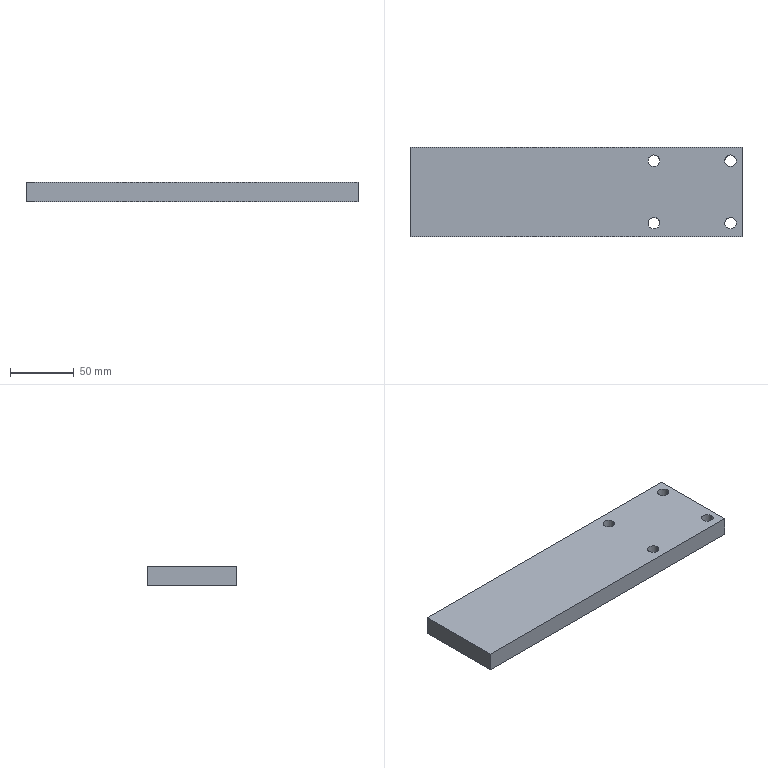Part | STEP file | Positioning_id466_x_t | 1 solid | 14 faces | box 260 x 70 x 15 mm | volume 269183 mm3 | cylinder 8 | plane 6 | commonest cylinder face diameters 9 x8
STEP:
#1=CARTESIAN_POINT('',(0.,0.,0.));
#2=DIRECTION('',(0.,0.,1.));
#3=DIRECTION('',(1.,0.,0.));
#4=AXIS2_PLACEMENT_3D('',#1,#2,#3);
#5=CARTESIAN_POINT('',(-826.502,-177.,373.532));
#6=VERTEX_POINT('',#5);
#7=CARTESIAN_POINT('',(-817.502,-177.,373.532));
#8=VERTEX_POINT('',#7);
#9=CARTESIAN_POINT('',(-822.002,-177.,373.532));
#10=DIRECTION('',(0.,0.,1.));
#11=DIRECTION('',(-1.,0.,0.));
#12=AXIS2_PLACEMENT_3D('',#9,#10,#11);
#13=CIRCLE('',#12,4.5);
#14=CARTESIAN_POINT('',(-822.002,-177.,293.532));
#15=DIRECTION('',(0.,0.,-1.));
#16=DIRECTION('',(1.,0.,0.));
#17=AXIS2_PLACEMENT_3D('',#14,#15,#16);
#18=CYLINDRICAL_SURFACE('',#17,4.5);
#19=CARTESIAN_POINT('',(3.142,-80.));
#20=DIRECTION('',(-1.,0.));
#21=VECTOR('',#20,1.);
#22=LINE('',#19,#21);
#23=(GEOMETRIC_REPRESENTATION_CONTEXT(2)PARAMETRIC_REPRESENTATION_CONTEXT()REPRESENTATION_CONTEXT('',''));
#24=DEFINITIONAL_REPRESENTATION('',(#22),#23);
#25=PCURVE('',#18,#24);
#26=CARTESIAN_POINT('',(-850.002,-164.,373.532));
#27=DIRECTION('',(0.,0.,1.));
#28=DIRECTION('',(0.,1.,0.));
#29=AXIS2_PLACEMENT_3D('',#26,#27,#28);
#30=PLANE('',#29);
#31=CARTESIAN_POINT('',(-13.,-28.));
#32=DIRECTION('',(0.,1.));
#33=AXIS2_PLACEMENT_2D('',#31,#32);
#34=CIRCLE('',#33,4.5);
#35=(GEOMETRIC_REPRESENTATION_CONTEXT(2)PARAMETRIC_REPRESENTATION_CONTEXT()REPRESENTATION_CONTEXT('',''));
#36=DEFINITIONAL_REPRESENTATION('',(#34),#35);
#37=PCURVE('',#30,#36);
#38=SURFACE_CURVE('',#13,(#25,#37),.PCURVE_S1.);
#39=EDGE_CURVE('',#6,#8,#38,.T.);
#40=ORIENTED_EDGE('',*,*,#39,.F.);
#41=CARTESIAN_POINT('',(-826.502,-177.,358.532));
#42=VERTEX_POINT('',#41);
#43=CARTESIAN_POINT('',(-826.502,-177.,358.532));
#44=DIRECTION('',(0.,0.,1.));
#45=VECTOR('',#44,1.);
#46=LINE('',#43,#45);
#47=CARTESIAN_POINT('',(3.142,-65.));
#48=DIRECTION('',(0.,-1.));
#49=VECTOR('',#48,1.);
#50=LINE('',#47,#49);
#51=(GEOMETRIC_REPRESENTATION_CONTEXT(2)PARAMETRIC_REPRESENTATION_CONTEXT()REPRESENTATION_CONTEXT('',''));
#52=DEFINITIONAL_REPRESENTATION('',(#50),#51);
#53=PCURVE('',#18,#52);
#54=CARTESIAN_POINT('',(-822.002,-177.,293.532));
#55=DIRECTION('',(0.,0.,-1.));
#56=DIRECTION('',(1.,0.,0.));
#57=AXIS2_PLACEMENT_3D('',#54,#55,#56);
#58=CYLINDRICAL_SURFACE('',#57,4.5);
#59=CARTESIAN_POINT('',(3.142,-65.));
#60=DIRECTION('',(0.,-1.));
#61=VECTOR('',#60,1.);
#62=LINE('',#59,#61);
#63=(GEOMETRIC_REPRESENTATION_CONTEXT(2)PARAMETRIC_REPRESENTATION_CONTEXT()REPRESENTATION_CONTEXT('',''));
#64=DEFINITIONAL_REPRESENTATION('',(#62),#63);
#65=PCURVE('',#58,#64);
#66=SURFACE_CURVE('',#46,(#53,#65),.PCURVE_S1.);
#67=EDGE_CURVE('',#42,#6,#66,.T.);
#68=ORIENTED_EDGE('',*,*,#67,.F.);
#69=CARTESIAN_POINT('',(-817.502,-177.,358.532));
#70=VERTEX_POINT('',#69);
#71=CARTESIAN_POINT('',(-822.002,-177.,358.532));
#72=DIRECTION('',(0.,0.,-1.));
#73=DIRECTION('',(-1.,0.,0.));
#74=AXIS2_PLACEMENT_3D('',#71,#72,#73);
#75=CIRCLE('',#74,4.5);
#76=CARTESIAN_POINT('',(-3.142,-65.));
#77=DIRECTION('',(1.,0.));
#78=VECTOR('',#77,1.);
#79=LINE('',#76,#78);
#80=(GEOMETRIC_REPRESENTATION_CONTEXT(2)PARAMETRIC_REPRESENTATION_CONTEXT()REPRESENTATION_CONTEXT('',''));
#81=DEFINITIONAL_REPRESENTATION('',(#79),#80);
#82=PCURVE('',#18,#81);
#83=CARTESIAN_POINT('',(-850.002,-164.,358.532));
#84=DIRECTION('',(0.,0.,-1.));
#85=DIRECTION('',(0.,-1.,0.));
#86=AXIS2_PLACEMENT_3D('',#83,#84,#85);
#87=PLANE('',#86);
#88=CARTESIAN_POINT('',(13.,-28.));
#89=DIRECTION('',(0.,1.));
#90=AXIS2_PLACEMENT_2D('',#88,#89);
#91=CIRCLE('',#90,4.5);
#92=(GEOMETRIC_REPRESENTATION_CONTEXT(2)PARAMETRIC_REPRESENTATION_CONTEXT()REPRESENTATION_CONTEXT('',''));
#93=DEFINITIONAL_REPRESENTATION('',(#91),#92);
#94=PCURVE('',#87,#93);
#95=SURFACE_CURVE('',#75,(#82,#94),.PCURVE_S1.);
#96=EDGE_CURVE('',#70,#42,#95,.T.);
#97=ORIENTED_EDGE('',*,*,#96,.F.);
#98=CARTESIAN_POINT('',(-817.502,-177.,358.532));
#99=DIRECTION('',(0.,0.,-1.));
#100=VECTOR('',#99,1.);
#101=LINE('',#98,#100);
#102=CARTESIAN_POINT('',(0.,-65.));
#103=DIRECTION('',(0.,1.));
#104=VECTOR('',#103,1.);
#105=LINE('',#102,#104);
#106=(GEOMETRIC_REPRESENTATION_CONTEXT(2)PARAMETRIC_REPRESENTATION_CONTEXT()REPRESENTATION_CONTEXT('',''));
#107=DEFINITIONAL_REPRESENTATION('',(#105),#106);
#108=PCURVE('',#18,#107);
#109=CARTESIAN_POINT('',(6.283,-65.));
#110=DIRECTION('',(0.,1.));
#111=VECTOR('',#110,1.);
#112=LINE('',#109,#111);
#113=(GEOMETRIC_REPRESENTATION_CONTEXT(2)PARAMETRIC_REPRESENTATION_CONTEXT()REPRESENTATION_CONTEXT('',''));
#114=DEFINITIONAL_REPRESENTATION('',(#112),#113);
#115=PCURVE('',#58,#114);
#116=SURFACE_CURVE('',#101,(#108,#115),.PCURVE_S1.);
#117=EDGE_CURVE('',#8,#70,#116,.T.);
#118=ORIENTED_EDGE('',*,*,#117,.F.);
#119=EDGE_LOOP('',(#40,#68,#97,#118));
#120=FACE_BOUND('',#119,.F.);
#121=ADVANCED_FACE('',(#120),#18,.F.);
#122=CARTESIAN_POINT('',(-826.502,-226.,373.532));
#123=VERTEX_POINT('',#122);
#124=CARTESIAN_POINT('',(-817.502,-226.,373.532));
#125=VERTEX_POINT('',#124);
#126=CARTESIAN_POINT('',(-822.002,-226.,373.532));
#127=DIRECTION('',(0.,0.,1.));
#128=DIRECTION('',(-1.,0.,0.));
#129=AXIS2_PLACEMENT_3D('',#126,#127,#128);
#130=CIRCLE('',#129,4.5);
#131=CARTESIAN_POINT('',(-822.002,-226.,293.532));
#132=DIRECTION('',(0.,0.,-1.));
#133=DIRECTION('',(1.,0.,0.));
#134=AXIS2_PLACEMENT_3D('',#131,#132,#133);
#135=CYLINDRICAL_SURFACE('',#134,4.5);
#136=CARTESIAN_POINT('',(3.142,-80.));
#137=DIRECTION('',(-1.,0.));
#138=VECTOR('',#137,1.);
#139=LINE('',#136,#138);
#140=(GEOMETRIC_REPRESENTATION_CONTEXT(2)PARAMETRIC_REPRESENTATION_CONTEXT()REPRESENTATION_CONTEXT('',''));
#141=DEFINITIONAL_REPRESENTATION('',(#139),#140);
#142=PCURVE('',#135,#141);
#143=CARTESIAN_POINT('',(-62.,-28.));
#144=DIRECTION('',(0.,1.));
#145=AXIS2_PLACEMENT_2D('',#143,#144);
#146=CIRCLE('',#145,4.5);
#147=(GEOMETRIC_REPRESENTATION_CONTEXT(2)PARAMETRIC_REPRESENTATION_CONTEXT()REPRESENTATION_CONTEXT('',''));
#148=DEFINITIONAL_REPRESENTATION('',(#146),#147);
#149=PCURVE('',#30,#148);
#150=SURFACE_CURVE('',#130,(#142,#149),.PCURVE_S1.);
#151=EDGE_CURVE('',#123,#125,#150,.T.);
#152=ORIENTED_EDGE('',*,*,#151,.F.);
#153=CARTESIAN_POINT('',(-826.502,-226.,358.532));
#154=VERTEX_POINT('',#153);
#155=CARTESIAN_POINT('',(-826.502,-226.,358.532));
#156=DIRECTION('',(0.,0.,-1.));
#157=VECTOR('',#156,1.);
#158=LINE('',#155,#157);
#159=CARTESIAN_POINT('',(3.142,-65.));
#160=DIRECTION('',(0.,1.));
#161=VECTOR('',#160,1.);
#162=LINE('',#159,#161);
#163=(GEOMETRIC_REPRESENTATION_CONTEXT(2)PARAMETRIC_REPRESENTATION_CONTEXT()REPRESENTATION_CONTEXT('',''));
#164=DEFINITIONAL_REPRESENTATION('',(#162),#163);
#165=PCURVE('',#135,#164);
#166=CARTESIAN_POINT('',(-822.002,-226.,293.532));
#167=DIRECTION('',(0.,0.,-1.));
#168=DIRECTION('',(1.,0.,0.));
#169=AXIS2_PLACEMENT_3D('',#166,#167,#168);
#170=CYLINDRICAL_SURFACE('',#169,4.5);
#171=CARTESIAN_POINT('',(3.142,-65.));
#172=DIRECTION('',(0.,1.));
#173=VECTOR('',#172,1.);
#174=LINE('',#171,#173);
#175=(GEOMETRIC_REPRESENTATION_CONTEXT(2)PARAMETRIC_REPRESENTATION_CONTEXT()REPRESENTATION_CONTEXT('',''));
#176=DEFINITIONAL_REPRESENTATION('',(#174),#175);
#177=PCURVE('',#170,#176);
#178=SURFACE_CURVE('',#158,(#165,#177),.PCURVE_S1.);
#179=EDGE_CURVE('',#123,#154,#178,.T.);
#180=ORIENTED_EDGE('',*,*,#179,.T.);
#181=CARTESIAN_POINT('',(-817.502,-226.,358.532));
#182=VERTEX_POINT('',#181);
#183=CARTESIAN_POINT('',(-822.002,-226.,358.532));
#184=DIRECTION('',(0.,0.,-1.));
#185=DIRECTION('',(-1.,0.,0.));
#186=AXIS2_PLACEMENT_3D('',#183,#184,#185);
#187=CIRCLE('',#186,4.5);
#188=CARTESIAN_POINT('',(-3.142,-65.));
#189=DIRECTION('',(1.,0.));
#190=VECTOR('',#189,1.);
#191=LINE('',#188,#190);
#192=(GEOMETRIC_REPRESENTATION_CONTEXT(2)PARAMETRIC_REPRESENTATION_CONTEXT()REPRESENTATION_CONTEXT('',''));
#193=DEFINITIONAL_REPRESENTATION('',(#191),#192);
#194=PCURVE('',#135,#193);
#195=CARTESIAN_POINT('',(62.,-28.));
#196=DIRECTION('',(0.,1.));
#197=AXIS2_PLACEMENT_2D('',#195,#196);
#198=CIRCLE('',#197,4.5);
#199=(GEOMETRIC_REPRESENTATION_CONTEXT(2)PARAMETRIC_REPRESENTATION_CONTEXT()REPRESENTATION_CONTEXT('',''));
#200=DEFINITIONAL_REPRESENTATION('',(#198),#199);
#201=PCURVE('',#87,#200);
#202=SURFACE_CURVE('',#187,(#194,#201),.PCURVE_S1.);
#203=EDGE_CURVE('',#182,#154,#202,.T.);
#204=ORIENTED_EDGE('',*,*,#203,.F.);
#205=CARTESIAN_POINT('',(-817.502,-226.,358.532));
#206=DIRECTION('',(0.,0.,1.));
#207=VECTOR('',#206,1.);
#208=LINE('',#205,#207);
#209=CARTESIAN_POINT('',(0.,-65.));
#210=DIRECTION('',(0.,-1.));
#211=VECTOR('',#210,1.);
#212=LINE('',#209,#211);
#213=(GEOMETRIC_REPRESENTATION_CONTEXT(2)PARAMETRIC_REPRESENTATION_CONTEXT()REPRESENTATION_CONTEXT('',''));
#214=DEFINITIONAL_REPRESENTATION('',(#212),#213);
#215=PCURVE('',#135,#214);
#216=CARTESIAN_POINT('',(6.283,-65.));
#217=DIRECTION('',(0.,-1.));
#218=VECTOR('',#217,1.);
#219=LINE('',#216,#218);
#220=(GEOMETRIC_REPRESENTATION_CONTEXT(2)PARAMETRIC_REPRESENTATION_CONTEXT()REPRESENTATION_CONTEXT('',''));
#221=DEFINITIONAL_REPRESENTATION('',(#219),#220);
#222=PCURVE('',#170,#221);
#223=SURFACE_CURVE('',#208,(#215,#222),.PCURVE_S1.);
#224=EDGE_CURVE('',#182,#125,#223,.T.);
#225=ORIENTED_EDGE('',*,*,#224,.T.);
#226=EDGE_LOOP('',(#152,#180,#204,#225));
#227=FACE_BOUND('',#226,.F.);
#228=ADVANCED_FACE('',(#227),#135,.F.);
#229=CARTESIAN_POINT('',(-766.502,-226.,373.532));
#230=VERTEX_POINT('',#229);
#231=CARTESIAN_POINT('',(-757.502,-226.,373.532));
#232=VERTEX_POINT('',#231);
#233=CARTESIAN_POINT('',(-762.002,-226.,373.532));
#234=DIRECTION('',(0.,0.,1.));
#235=DIRECTION('',(-1.,0.,0.));
#236=AXIS2_PLACEMENT_3D('',#233,#234,#235);
#237=CIRCLE('',#236,4.5);
#238=CARTESIAN_POINT('',(-762.002,-226.,293.532));
#239=DIRECTION('',(0.,0.,-1.));
#240=DIRECTION('',(1.,0.,0.));
#241=AXIS2_PLACEMENT_3D('',#238,#239,#240);
#242=CYLINDRICAL_SURFACE('',#241,4.5);
#243=CARTESIAN_POINT('',(3.142,-80.));
#244=DIRECTION('',(-1.,0.));
#245=VECTOR('',#244,1.);
#246=LINE('',#243,#245);
#247=(GEOMETRIC_REPRESENTATION_CONTEXT(2)PARAMETRIC_REPRESENTATION_CONTEXT()REPRESENTATION_CONTEXT('',''));
#248=DEFINITIONAL_REPRESENTATION('',(#246),#247);
#249=PCURVE('',#242,#248);
#250=CARTESIAN_POINT('',(-62.,-88.));
#251=DIRECTION('',(0.,1.));
#252=AXIS2_PLACEMENT_2D('',#250,#251);
#253=CIRCLE('',#252,4.5);
#254=(GEOMETRIC_REPRESENTATION_CONTEXT(2)PARAMETRIC_REPRESENTATION_CONTEXT()REPRESENTATION_CONTEXT('',''));
#255=DEFINITIONAL_REPRESENTATION('',(#253),#254);
#256=PCURVE('',#30,#255);
#257=SURFACE_CURVE('',#237,(#249,#256),.PCURVE_S1.);
#258=EDGE_CURVE('',#230,#232,#257,.T.);
#259=ORIENTED_EDGE('',*,*,#258,.F.);
#260=CARTESIAN_POINT('',(-766.502,-226.,358.532));
#261=VERTEX_POINT('',#260);
#262=CARTESIAN_POINT('',(-766.502,-226.,358.532));
#263=DIRECTION('',(0.,0.,1.));
#264=VECTOR('',#263,1.);
#265=LINE('',#262,#264);
#266=CARTESIAN_POINT('',(3.142,-65.));
#267=DIRECTION('',(0.,-1.));
#268=VECTOR('',#267,1.);
#269=LINE('',#266,#268);
#270=(GEOMETRIC_REPRESENTATION_CONTEXT(2)PARAMETRIC_REPRESENTATION_CONTEXT()REPRESENTATION_CONTEXT('',''));
#271=DEFINITIONAL_REPRESENTATION('',(#269),#270);
#272=PCURVE('',#242,#271);
#273=CARTESIAN_POINT('',(-762.002,-226.,293.532));
#274=DIRECTION('',(0.,0.,-1.));
#275=DIRECTION('',(1.,0.,0.));
#276=AXIS2_PLACEMENT_3D('',#273,#274,#275);
#277=CYLINDRICAL_SURFACE('',#276,4.5);
#278=CARTESIAN_POINT('',(3.142,-65.));
#279=DIRECTION('',(0.,-1.));
#280=VECTOR('',#279,1.);
#281=LINE('',#278,#280);
#282=(GEOMETRIC_REPRESENTATION_CONTEXT(2)PARAMETRIC_REPRESENTATION_CONTEXT()REPRESENTATION_CONTEXT('',''));
#283=DEFINITIONAL_REPRESENTATION('',(#281),#282);
#284=PCURVE('',#277,#283);
#285=SURFACE_CURVE('',#265,(#272,#284),.PCURVE_S1.);
#286=EDGE_CURVE('',#261,#230,#285,.T.);
#287=ORIENTED_EDGE('',*,*,#286,.F.);
#288=CARTESIAN_POINT('',(-757.502,-226.,358.532));
#289=VERTEX_POINT('',#288);
#290=CARTESIAN_POINT('',(-762.002,-226.,358.532));
#291=DIRECTION('',(0.,0.,-1.));
#292=DIRECTION('',(-1.,0.,0.));
#293=AXIS2_PLACEMENT_3D('',#290,#291,#292);
#294=CIRCLE('',#293,4.5);
#295=CARTESIAN_POINT('',(-3.142,-65.));
#296=DIRECTION('',(1.,0.));
#297=VECTOR('',#296,1.);
#298=LINE('',#295,#297);
#299=(GEOMETRIC_REPRESENTATION_CONTEXT(2)PARAMETRIC_REPRESENTATION_CONTEXT()REPRESENTATION_CONTEXT('',''));
#300=DEFINITIONAL_REPRESENTATION('',(#298),#299);
#301=PCURVE('',#242,#300);
#302=CARTESIAN_POINT('',(62.,-88.));
#303=DIRECTION('',(0.,1.));
#304=AXIS2_PLACEMENT_2D('',#302,#303);
#305=CIRCLE('',#304,4.5);
#306=(GEOMETRIC_REPRESENTATION_CONTEXT(2)PARAMETRIC_REPRESENTATION_CONTEXT()REPRESENTATION_CONTEXT('',''));
#307=DEFINITIONAL_REPRESENTATION('',(#305),#306);
#308=PCURVE('',#87,#307);
#309=SURFACE_CURVE('',#294,(#301,#308),.PCURVE_S1.);
#310=EDGE_CURVE('',#289,#261,#309,.T.);
#311=ORIENTED_EDGE('',*,*,#310,.F.);
#312=CARTESIAN_POINT('',(-757.502,-226.,358.532));
#313=DIRECTION('',(0.,0.,-1.));
#314=VECTOR('',#313,1.);
#315=LINE('',#312,#314);
#316=CARTESIAN_POINT('',(0.,-65.));
#317=DIRECTION('',(0.,1.));
#318=VECTOR('',#317,1.);
#319=LINE('',#316,#318);
#320=(GEOMETRIC_REPRESENTATION_CONTEXT(2)PARAMETRIC_REPRESENTATION_CONTEXT()REPRESENTATION_CONTEXT('',''));
#321=DEFINITIONAL_REPRESENTATION('',(#319),#320);
#322=PCURVE('',#242,#321);
#323=CARTESIAN_POINT('',(6.283,-65.));
#324=DIRECTION('',(0.,1.));
#325=VECTOR('',#324,1.);
#326=LINE('',#323,#325);
#327=(GEOMETRIC_REPRESENTATION_CONTEXT(2)PARAMETRIC_REPRESENTATION_CONTEXT()REPRESENTATION_CONTEXT('',''));
#328=DEFINITIONAL_REPRESENTATION('',(#326),#327);
#329=PCURVE('',#277,#328);
#330=SURFACE_CURVE('',#315,(#322,#329),.PCURVE_S1.);
#331=EDGE_CURVE('',#232,#289,#330,.T.);
#332=ORIENTED_EDGE('',*,*,#331,.F.);
#333=EDGE_LOOP('',(#259,#287,#311,#332));
#334=FACE_BOUND('',#333,.F.);
#335=ADVANCED_FACE('',(#334),#242,.F.);
#336=CARTESIAN_POINT('',(-766.502,-177.,373.532));
#337=VERTEX_POINT('',#336);
#338=CARTESIAN_POINT('',(-757.502,-177.,373.532));
#339=VERTEX_POINT('',#338);
#340=CARTESIAN_POINT('',(-762.002,-177.,373.532));
#341=DIRECTION('',(0.,0.,1.));
#342=DIRECTION('',(-1.,0.,0.));
#343=AXIS2_PLACEMENT_3D('',#340,#341,#342);
#344=CIRCLE('',#343,4.5);
#345=CARTESIAN_POINT('',(-762.002,-177.,293.532));
#346=DIRECTION('',(0.,0.,-1.));
#347=DIRECTION('',(1.,0.,0.));
#348=AXIS2_PLACEMENT_3D('',#345,#346,#347);
#349=CYLINDRICAL_SURFACE('',#348,4.5);
#350=CARTESIAN_POINT('',(3.142,-80.));
#351=DIRECTION('',(-1.,0.));
#352=VECTOR('',#351,1.);
#353=LINE('',#350,#352);
#354=(GEOMETRIC_REPRESENTATION_CONTEXT(2)PARAMETRIC_REPRESENTATION_CONTEXT()REPRESENTATION_CONTEXT('',''));
#355=DEFINITIONAL_REPRESENTATION('',(#353),#354);
#356=PCURVE('',#349,#355);
#357=CARTESIAN_POINT('',(-13.,-88.));
#358=DIRECTION('',(0.,1.));
#359=AXIS2_PLACEMENT_2D('',#357,#358);
#360=CIRCLE('',#359,4.5);
#361=(GEOMETRIC_REPRESENTATION_CONTEXT(2)PARAMETRIC_REPRESENTATION_CONTEXT()REPRESENTATION_CONTEXT('',''));
#362=DEFINITIONAL_REPRESENTATION('',(#360),#361);
#363=PCURVE('',#30,#362);
#364=SURFACE_CURVE('',#344,(#356,#363),.PCURVE_S1.);
#365=EDGE_CURVE('',#337,#339,#364,.T.);
#366=ORIENTED_EDGE('',*,*,#365,.F.);
#367=CARTESIAN_POINT('',(-766.502,-177.,358.532));
#368=VERTEX_POINT('',#367);
#369=CARTESIAN_POINT('',(-766.502,-177.,358.532));
#370=DIRECTION('',(0.,0.,-1.));
#371=VECTOR('',#370,1.);
#372=LINE('',#369,#371);
#373=CARTESIAN_POINT('',(3.142,-65.));
#374=DIRECTION('',(0.,1.));
#375=VECTOR('',#374,1.);
#376=LINE('',#373,#375);
#377=(GEOMETRIC_REPRESENTATION_CONTEXT(2)PARAMETRIC_REPRESENTATION_CONTEXT()REPRESENTATION_CONTEXT('',''));
#378=DEFINITIONAL_REPRESENTATION('',(#376),#377);
#379=PCURVE('',#349,#378);
#380=CARTESIAN_POINT('',(-762.002,-177.,293.532));
#381=DIRECTION('',(0.,0.,-1.));
#382=DIRECTION('',(1.,0.,0.));
#383=AXIS2_PLACEMENT_3D('',#380,#381,#382);
#384=CYLINDRICAL_SURFACE('',#383,4.5);
#385=CARTESIAN_POINT('',(3.142,-65.));
#386=DIRECTION('',(0.,1.));
#387=VECTOR('',#386,1.);
#388=LINE('',#385,#387);
#389=(GEOMETRIC_REPRESENTATION_CONTEXT(2)PARAMETRIC_REPRESENTATION_CONTEXT()REPRESENTATION_CONTEXT('',''));
#390=DEFINITIONAL_REPRESENTATION('',(#388),#389);
#391=PCURVE('',#384,#390);
#392=SURFACE_CURVE('',#372,(#379,#391),.PCURVE_S1.);
#393=EDGE_CURVE('',#337,#368,#392,.T.);
#394=ORIENTED_EDGE('',*,*,#393,.T.);
#395=CARTESIAN_POINT('',(-757.502,-177.,358.532));
#396=VERTEX_POINT('',#395);
#397=CARTESIAN_POINT('',(-762.002,-177.,358.532));
#398=DIRECTION('',(0.,0.,-1.));
#399=DIRECTION('',(-1.,0.,0.));
#400=AXIS2_PLACEMENT_3D('',#397,#398,#399);
#401=CIRCLE('',#400,4.5);
#402=CARTESIAN_POINT('',(-3.142,-65.));
#403=DIRECTION('',(1.,0.));
#404=VECTOR('',#403,1.);
#405=LINE('',#402,#404);
#406=(GEOMETRIC_REPRESENTATION_CONTEXT(2)PARAMETRIC_REPRESENTATION_CONTEXT()REPRESENTATION_CONTEXT('',''));
#407=DEFINITIONAL_REPRESENTATION('',(#405),#406);
#408=PCURVE('',#349,#407);
#409=CARTESIAN_POINT('',(13.,-88.));
#410=DIRECTION('',(0.,1.));
#411=AXIS2_PLACEMENT_2D('',#409,#410);
#412=CIRCLE('',#411,4.5);
#413=(GEOMETRIC_REPRESENTATION_CONTEXT(2)PARAMETRIC_REPRESENTATION_CONTEXT()REPRESENTATION_CONTEXT('',''));
#414=DEFINITIONAL_REPRESENTATION('',(#412),#413);
#415=PCURVE('',#87,#414);
#416=SURFACE_CURVE('',#401,(#408,#415),.PCURVE_S1.);
#417=EDGE_CURVE('',#396,#368,#416,.T.);
#418=ORIENTED_EDGE('',*,*,#417,.F.);
#419=CARTESIAN_POINT('',(-757.502,-177.,358.532));
#420=DIRECTION('',(0.,0.,1.));
#421=VECTOR('',#420,1.);
#422=LINE('',#419,#421);
#423=CARTESIAN_POINT('',(0.,-65.));
#424=DIRECTION('',(0.,-1.));
#425=VECTOR('',#424,1.);
#426=LINE('',#423,#425);
#427=(GEOMETRIC_REPRESENTATION_CONTEXT(2)PARAMETRIC_REPRESENTATION_CONTEXT()REPRESENTATION_CONTEXT('',''));
#428=DEFINITIONAL_REPRESENTATION('',(#426),#427);
#429=PCURVE('',#349,#428);
#430=CARTESIAN_POINT('',(6.283,-65.));
#431=DIRECTION('',(0.,-1.));
#432=VECTOR('',#431,1.);
#433=LINE('',#430,#432);
#434=(GEOMETRIC_REPRESENTATION_CONTEXT(2)PARAMETRIC_REPRESENTATION_CONTEXT()REPRESENTATION_CONTEXT('',''));
#435=DEFINITIONAL_REPRESENTATION('',(#433),#434);
#436=PCURVE('',#384,#435);
#437=SURFACE_CURVE('',#422,(#429,#436),.PCURVE_S1.);
#438=EDGE_CURVE('',#396,#339,#437,.T.);
#439=ORIENTED_EDGE('',*,*,#438,.T.);
#440=EDGE_LOOP('',(#366,#394,#418,#439));
#441=FACE_BOUND('',#440,.F.);
#442=ADVANCED_FACE('',(#441),#349,.F.);
#443=CARTESIAN_POINT('',(-1013.002,-236.5,358.532));
#444=VERTEX_POINT('',#443);
#445=CARTESIAN_POINT('',(-1013.002,-236.5,373.532));
#446=VERTEX_POINT('',#445);
#447=CARTESIAN_POINT('',(-1013.002,-236.5,358.532));
#448=DIRECTION('',(0.,0.,1.));
#449=VECTOR('',#448,1.);
#450=LINE('',#447,#449);
#451=CARTESIAN_POINT('',(-1013.002,95.25,13.032));
#452=DIRECTION('',(1.,0.,0.));
#453=DIRECTION('',(0.,-1.,0.));
#454=AXIS2_PLACEMENT_3D('',#451,#452,#453);
#455=PLANE('',#454);
#456=CARTESIAN_POINT('',(331.75,-345.5));
#457=DIRECTION('',(0.,-1.));
#458=VECTOR('',#457,1.);
#459=LINE('',#456,#458);
#460=(GEOMETRIC_REPRESENTATION_CONTEXT(2)PARAMETRIC_REPRESENTATION_CONTEXT()REPRESENTATION_CONTEXT('',''));
#461=DEFINITIONAL_REPRESENTATION('',(#459),#460);
#462=PCURVE('',#455,#461);
#463=CARTESIAN_POINT('',(-850.002,-236.5,388.532));
#464=DIRECTION('',(0.,-1.,0.));
#465=DIRECTION('',(-1.,0.,0.));
#466=AXIS2_PLACEMENT_3D('',#463,#464,#465);
#467=PLANE('',#466);
#468=CARTESIAN_POINT('',(163.,30.));
#469=DIRECTION('',(0.,-1.));
#470=VECTOR('',#469,1.);
#471=LINE('',#468,#470);
#472=(GEOMETRIC_REPRESENTATION_CONTEXT(2)PARAMETRIC_REPRESENTATION_CONTEXT()REPRESENTATION_CONTEXT('',''));
#473=DEFINITIONAL_REPRESENTATION('',(#471),#472);
#474=PCURVE('',#467,#473);
#475=SURFACE_CURVE('',#450,(#462,#474),.PCURVE_S1.);
#476=EDGE_CURVE('',#444,#446,#475,.T.);
#477=ORIENTED_EDGE('',*,*,#476,.T.);
#478=CARTESIAN_POINT('',(-1013.002,-166.5,373.532));
#479=VERTEX_POINT('',#478);
#480=CARTESIAN_POINT('',(-1013.002,-236.5,373.532));
#481=DIRECTION('',(0.,1.,0.));
#482=VECTOR('',#481,1.);
#483=LINE('',#480,#482);
#484=CARTESIAN_POINT('',(331.75,-360.5));
#485=DIRECTION('',(-1.,0.));
#486=VECTOR('',#485,1.);
#487=LINE('',#484,#486);
#488=(GEOMETRIC_REPRESENTATION_CONTEXT(2)PARAMETRIC_REPRESENTATION_CONTEXT()REPRESENTATION_CONTEXT('',''));
#489=DEFINITIONAL_REPRESENTATION('',(#487),#488);
#490=PCURVE('',#455,#489);
#491=CARTESIAN_POINT('',(-72.5,163.));
#492=DIRECTION('',(1.,0.));
#493=VECTOR('',#492,1.);
#494=LINE('',#491,#493);
#495=(GEOMETRIC_REPRESENTATION_CONTEXT(2)PARAMETRIC_REPRESENTATION_CONTEXT()REPRESENTATION_CONTEXT('',''));
#496=DEFINITIONAL_REPRESENTATION('',(#494),#495);
#497=PCURVE('',#30,#496);
#498=SURFACE_CURVE('',#483,(#490,#497),.PCURVE_S1.);
#499=EDGE_CURVE('',#446,#479,#498,.T.);
#500=ORIENTED_EDGE('',*,*,#499,.T.);
#501=CARTESIAN_POINT('',(-1013.002,-166.5,358.532));
#502=VERTEX_POINT('',#501);
#503=CARTESIAN_POINT('',(-1013.002,-166.5,373.532));
#504=DIRECTION('',(0.,0.,-1.));
#505=VECTOR('',#504,1.);
#506=LINE('',#503,#505);
#507=CARTESIAN_POINT('',(261.75,-360.5));
#508=DIRECTION('',(0.,1.));
#509=VECTOR('',#508,1.);
#510=LINE('',#507,#509);
#511=(GEOMETRIC_REPRESENTATION_CONTEXT(2)PARAMETRIC_REPRESENTATION_CONTEXT()REPRESENTATION_CONTEXT('',''));
#512=DEFINITIONAL_REPRESENTATION('',(#510),#511);
#513=PCURVE('',#455,#512);
#514=CARTESIAN_POINT('',(-850.002,-166.5,388.532));
#515=DIRECTION('',(0.,1.,0.));
#516=DIRECTION('',(1.,0.,0.));
#517=AXIS2_PLACEMENT_3D('',#514,#515,#516);
#518=PLANE('',#517);
#519=CARTESIAN_POINT('',(-163.,15.));
#520=DIRECTION('',(0.,1.));
#521=VECTOR('',#520,1.);
#522=LINE('',#519,#521);
#523=(GEOMETRIC_REPRESENTATION_CONTEXT(2)PARAMETRIC_REPRESENTATION_CONTEXT()REPRESENTATION_CONTEXT('',''));
#524=DEFINITIONAL_REPRESENTATION('',(#522),#523);
#525=PCURVE('',#518,#524);
#526=SURFACE_CURVE('',#506,(#513,#525),.PCURVE_S1.);
#527=EDGE_CURVE('',#479,#502,#526,.T.);
#528=ORIENTED_EDGE('',*,*,#527,.T.);
#529=CARTESIAN_POINT('',(-1013.002,-166.5,358.532));
#530=DIRECTION('',(0.,-1.,0.));
#531=VECTOR('',#530,1.);
#532=LINE('',#529,#531);
#533=CARTESIAN_POINT('',(261.75,-345.5));
#534=DIRECTION('',(1.,0.));
#535=VECTOR('',#534,1.);
#536=LINE('',#533,#535);
#537=(GEOMETRIC_REPRESENTATION_CONTEXT(2)PARAMETRIC_REPRESENTATION_CONTEXT()REPRESENTATION_CONTEXT('',''));
#538=DEFINITIONAL_REPRESENTATION('',(#536),#537);
#539=PCURVE('',#455,#538);
#540=CARTESIAN_POINT('',(2.5,163.));
#541=DIRECTION('',(1.,0.));
#542=VECTOR('',#541,1.);
#543=LINE('',#540,#542);
#544=(GEOMETRIC_REPRESENTATION_CONTEXT(2)PARAMETRIC_REPRESENTATION_CONTEXT()REPRESENTATION_CONTEXT('',''));
#545=DEFINITIONAL_REPRESENTATION('',(#543),#544);
#546=PCURVE('',#87,#545);
#547=SURFACE_CURVE('',#532,(#539,#546),.PCURVE_S1.);
#548=EDGE_CURVE('',#502,#444,#547,.T.);
#549=ORIENTED_EDGE('',*,*,#548,.T.);
#550=EDGE_LOOP('',(#477,#500,#528,#549));
#551=FACE_BOUND('',#550,.T.);
#552=ADVANCED_FACE('',(#551),#455,.F.);
#553=CARTESIAN_POINT('',(-753.002,-166.5,373.532));
#554=VERTEX_POINT('',#553);
#555=CARTESIAN_POINT('',(-753.002,-166.5,358.532));
#556=VERTEX_POINT('',#555);
#557=CARTESIAN_POINT('',(-753.002,-166.5,373.532));
#558=DIRECTION('',(0.,0.,-1.));
#559=VECTOR('',#558,1.);
#560=LINE('',#557,#559);
#561=CARTESIAN_POINT('',(-753.002,-164.,388.532));
#562=DIRECTION('',(1.,0.,0.));
#563=DIRECTION('',(0.,-1.,0.));
#564=AXIS2_PLACEMENT_3D('',#561,#562,#563);
#565=PLANE('',#564);
#566=CARTESIAN_POINT('',(2.5,15.));
#567=DIRECTION('',(0.,1.));
#568=VECTOR('',#567,1.);
#569=LINE('',#566,#568);
#570=(GEOMETRIC_REPRESENTATION_CONTEXT(2)PARAMETRIC_REPRESENTATION_CONTEXT()REPRESENTATION_CONTEXT('',''));
#571=DEFINITIONAL_REPRESENTATION('',(#569),#570);
#572=PCURVE('',#565,#571);
#573=CARTESIAN_POINT('',(97.,15.));
#574=DIRECTION('',(0.,1.));
#575=VECTOR('',#574,1.);
#576=LINE('',#573,#575);
#577=(GEOMETRIC_REPRESENTATION_CONTEXT(2)PARAMETRIC_REPRESENTATION_CONTEXT()REPRESENTATION_CONTEXT('',''));
#578=DEFINITIONAL_REPRESENTATION('',(#576),#577);
#579=PCURVE('',#518,#578);
#580=SURFACE_CURVE('',#560,(#572,#579),.PCURVE_S1.);
#581=EDGE_CURVE('',#554,#556,#580,.T.);
#582=ORIENTED_EDGE('',*,*,#581,.F.);
#583=CARTESIAN_POINT('',(-753.002,-236.5,373.532));
#584=VERTEX_POINT('',#583);
#585=CARTESIAN_POINT('',(-753.002,-166.5,373.532));
#586=DIRECTION('',(0.,-1.,0.));
#587=VECTOR('',#586,1.);
#588=LINE('',#585,#587);
#589=CARTESIAN_POINT('',(2.5,15.));
#590=DIRECTION('',(1.,0.));
#591=VECTOR('',#590,1.);
#592=LINE('',#589,#591);
#593=(GEOMETRIC_REPRESENTATION_CONTEXT(2)PARAMETRIC_REPRESENTATION_CONTEXT()REPRESENTATION_CONTEXT('',''));
#594=DEFINITIONAL_REPRESENTATION('',(#592),#593);
#595=PCURVE('',#565,#594);
#596=CARTESIAN_POINT('',(-2.5,-97.));
#597=DIRECTION('',(-1.,0.));
#598=VECTOR('',#597,1.);
#599=LINE('',#596,#598);
#600=(GEOMETRIC_REPRESENTATION_CONTEXT(2)PARAMETRIC_REPRESENTATION_CONTEXT()REPRESENTATION_CONTEXT('',''));
#601=DEFINITIONAL_REPRESENTATION('',(#599),#600);
#602=PCURVE('',#30,#601);
#603=SURFACE_CURVE('',#588,(#595,#602),.PCURVE_S1.);
#604=EDGE_CURVE('',#554,#584,#603,.T.);
#605=ORIENTED_EDGE('',*,*,#604,.T.);
#606=CARTESIAN_POINT('',(-753.002,-236.5,358.532));
#607=VERTEX_POINT('',#606);
#608=CARTESIAN_POINT('',(-753.002,-236.5,373.532));
#609=DIRECTION('',(0.,0.,-1.));
#610=VECTOR('',#609,1.);
#611=LINE('',#608,#610);
#612=CARTESIAN_POINT('',(72.5,15.));
#613=DIRECTION('',(0.,1.));
#614=VECTOR('',#613,1.);
#615=LINE('',#612,#614);
#616=(GEOMETRIC_REPRESENTATION_CONTEXT(2)PARAMETRIC_REPRESENTATION_CONTEXT()REPRESENTATION_CONTEXT('',''));
#617=DEFINITIONAL_REPRESENTATION('',(#615),#616);
#618=PCURVE('',#565,#617);
#619=CARTESIAN_POINT('',(-97.,15.));
#620=DIRECTION('',(0.,1.));
#621=VECTOR('',#620,1.);
#622=LINE('',#619,#621);
#623=(GEOMETRIC_REPRESENTATION_CONTEXT(2)PARAMETRIC_REPRESENTATION_CONTEXT()REPRESENTATION_CONTEXT('',''));
#624=DEFINITIONAL_REPRESENTATION('',(#622),#623);
#625=PCURVE('',#467,#624);
#626=SURFACE_CURVE('',#611,(#618,#625),.PCURVE_S1.);
#627=EDGE_CURVE('',#584,#607,#626,.T.);
#628=ORIENTED_EDGE('',*,*,#627,.T.);
#629=CARTESIAN_POINT('',(-753.002,-166.5,358.532));
#630=DIRECTION('',(0.,-1.,0.));
#631=VECTOR('',#630,1.);
#632=LINE('',#629,#631);
#633=CARTESIAN_POINT('',(2.5,30.));
#634=DIRECTION('',(1.,0.));
#635=VECTOR('',#634,1.);
#636=LINE('',#633,#635);
#637=(GEOMETRIC_REPRESENTATION_CONTEXT(2)PARAMETRIC_REPRESENTATION_CONTEXT()REPRESENTATION_CONTEXT('',''));
#638=DEFINITIONAL_REPRESENTATION('',(#636),#637);
#639=PCURVE('',#565,#638);
#640=CARTESIAN_POINT('',(2.5,-97.));
#641=DIRECTION('',(1.,0.));
#642=VECTOR('',#641,1.);
#643=LINE('',#640,#642);
#644=(GEOMETRIC_REPRESENTATION_CONTEXT(2)PARAMETRIC_REPRESENTATION_CONTEXT()REPRESENTATION_CONTEXT('',''));
#645=DEFINITIONAL_REPRESENTATION('',(#643),#644);
#646=PCURVE('',#87,#645);
#647=SURFACE_CURVE('',#632,(#639,#646),.PCURVE_S1.);
#648=EDGE_CURVE('',#556,#607,#647,.T.);
#649=ORIENTED_EDGE('',*,*,#648,.F.);
#650=EDGE_LOOP('',(#582,#605,#628,#649));
#651=FACE_BOUND('',#650,.T.);
#652=ADVANCED_FACE('',(#651),#565,.T.);
#653=CARTESIAN_POINT('',(-753.002,-166.5,373.532));
#654=DIRECTION('',(-1.,0.,0.));
#655=VECTOR('',#654,1.);
#656=LINE('',#653,#655);
#657=CARTESIAN_POINT('',(97.,15.));
#658=DIRECTION('',(-1.,0.));
#659=VECTOR('',#658,1.);
#660=LINE('',#657,#659);
#661=(GEOMETRIC_REPRESENTATION_CONTEXT(2)PARAMETRIC_REPRESENTATION_CONTEXT()REPRESENTATION_CONTEXT('',''));
#662=DEFINITIONAL_REPRESENTATION('',(#660),#661);
#663=PCURVE('',#518,#662);
#664=CARTESIAN_POINT('',(-2.5,-97.));
#665=DIRECTION('',(0.,1.));
#666=VECTOR('',#665,1.);
#667=LINE('',#664,#666);
#668=(GEOMETRIC_REPRESENTATION_CONTEXT(2)PARAMETRIC_REPRESENTATION_CONTEXT()REPRESENTATION_CONTEXT('',''));
#669=DEFINITIONAL_REPRESENTATION('',(#667),#668);
#670=PCURVE('',#30,#669);
#671=SURFACE_CURVE('',#656,(#663,#670),.PCURVE_S1.);
#672=EDGE_CURVE('',#554,#479,#671,.T.);
#673=ORIENTED_EDGE('',*,*,#672,.F.);
#674=ORIENTED_EDGE('',*,*,#581,.T.);
#675=CARTESIAN_POINT('',(-1013.002,-166.5,358.532));
#676=DIRECTION('',(1.,0.,0.));
#677=VECTOR('',#676,1.);
#678=LINE('',#675,#677);
#679=CARTESIAN_POINT('',(-163.,30.));
#680=DIRECTION('',(1.,0.));
#681=VECTOR('',#680,1.);
#682=LINE('',#679,#681);
#683=(GEOMETRIC_REPRESENTATION_CONTEXT(2)PARAMETRIC_REPRESENTATION_CONTEXT()REPRESENTATION_CONTEXT('',''));
#684=DEFINITIONAL_REPRESENTATION('',(#682),#683);
#685=PCURVE('',#518,#684);
#686=CARTESIAN_POINT('',(2.5,163.));
#687=DIRECTION('',(0.,-1.));
#688=VECTOR('',#687,1.);
#689=LINE('',#686,#688);
#690=(GEOMETRIC_REPRESENTATION_CONTEXT(2)PARAMETRIC_REPRESENTATION_CONTEXT()REPRESENTATION_CONTEXT('',''));
#691=DEFINITIONAL_REPRESENTATION('',(#689),#690);
#692=PCURVE('',#87,#691);
#693=SURFACE_CURVE('',#678,(#685,#692),.PCURVE_S1.);
#694=EDGE_CURVE('',#502,#556,#693,.T.);
#695=ORIENTED_EDGE('',*,*,#694,.F.);
#696=ORIENTED_EDGE('',*,*,#527,.F.);
#697=EDGE_LOOP('',(#673,#674,#695,#696));
#698=FACE_BOUND('',#697,.T.);
#699=ADVANCED_FACE('',(#698),#518,.T.);
#700=ORIENTED_EDGE('',*,*,#365,.F.);
#701=CARTESIAN_POINT('',(-757.502,-177.,373.532));
#702=CARTESIAN_POINT('',(-757.502,-172.5,373.532));
#703=CARTESIAN_POINT('',(-762.002,-170.25,373.532));
#704=CARTESIAN_POINT('',(-766.502,-172.5,373.532));
#705=CARTESIAN_POINT('',(-766.502,-177.,373.532));
#706=(BOUNDED_CURVE()B_SPLINE_CURVE(4,(#701,#702,#703,#704,#705),.UNSPECIFIED.,.F.,.F.)B_SPLINE_CURVE_WITH_KNOTS((5,5),(0.,1.),.PIECEWISE_BEZIER_KNOTS.)CURVE()GEOMETRIC_REPRESENTATION_ITEM()RATIONAL_B_SPLINE_CURVE((1.,0.7071,0.6667,0.7071,1.))REPRESENTATION_ITEM(''));
#707=CARTESIAN_POINT('',(-13.,-92.5));
#708=CARTESIAN_POINT('',(-8.5,-92.5));
#709=CARTESIAN_POINT('',(-6.25,-88.));
#710=CARTESIAN_POINT('',(-8.5,-83.5));
#711=CARTESIAN_POINT('',(-13.,-83.5));
#712=(BOUNDED_CURVE()B_SPLINE_CURVE(4,(#707,#708,#709,#710,#711),.UNSPECIFIED.,.F.,.F.)B_SPLINE_CURVE_WITH_KNOTS((5,5),(0.,1.),.PIECEWISE_BEZIER_KNOTS.)CURVE()GEOMETRIC_REPRESENTATION_ITEM()RATIONAL_B_SPLINE_CURVE((1.,0.7071,0.6667,0.7071,1.))REPRESENTATION_ITEM(''));
#713=(GEOMETRIC_REPRESENTATION_CONTEXT(2)PARAMETRIC_REPRESENTATION_CONTEXT()REPRESENTATION_CONTEXT('',''));
#714=DEFINITIONAL_REPRESENTATION('',(#712),#713);
#715=PCURVE('',#30,#714);
#716=CARTESIAN_POINT('',(6.283,-80.));
#717=CARTESIAN_POINT('',(6.24,-80.));
#718=CARTESIAN_POINT('',(6.153,-80.));
#719=CARTESIAN_POINT('',(6.02,-80.));
#720=CARTESIAN_POINT('',(5.883,-80.));
#721=CARTESIAN_POINT('',(5.744,-80.));
#722=CARTESIAN_POINT('',(5.602,-80.));
#723=CARTESIAN_POINT('',(5.457,-80.));
#724=CARTESIAN_POINT('',(5.311,-80.));
#725=CARTESIAN_POINT('',(5.163,-80.));
#726=CARTESIAN_POINT('',(5.013,-80.));
#727=CARTESIAN_POINT('',(4.863,-80.));
#728=CARTESIAN_POINT('',(4.712,-80.));
#729=CARTESIAN_POINT('',(4.562,-80.));
#730=CARTESIAN_POINT('',(4.412,-80.));
#731=CARTESIAN_POINT('',(4.262,-80.));
#732=CARTESIAN_POINT('',(4.114,-80.));
#733=CARTESIAN_POINT('',(3.968,-80.));
#734=CARTESIAN_POINT('',(3.823,-80.));
#735=CARTESIAN_POINT('',(3.681,-80.));
#736=CARTESIAN_POINT('',(3.542,-80.));
#737=CARTESIAN_POINT('',(3.405,-80.));
#738=CARTESIAN_POINT('',(3.271,-80.));
#739=CARTESIAN_POINT('',(3.184,-80.));
#740=CARTESIAN_POINT('',(3.142,-80.));
#741=B_SPLINE_CURVE_WITH_KNOTS('',3,(#716,#717,#718,#719,#720,#721,#722,#723,#724,#725,#726,#727,#728,#729,#730,#731,#732,#733,#734,#735,#736,#737,#738,#739,#740),.UNSPECIFIED.,.F.,.F.,(4,1,1,1,1,1,1,1,1,1,1,1,1,1,1,1,1,1,1,1,1,1,4),(0.,0.04545,0.09091,0.1364,0.1818,0.2273,0.2727,0.3182,0.3636,0.4091,0.4545,0.5,0.5455,0.5909,0.6364,0.6818,0.7273,0.7727,0.8182,0.8636,0.9091,0.9545,1.),.QUASI_UNIFORM_KNOTS.);
#742=(GEOMETRIC_REPRESENTATION_CONTEXT(2)PARAMETRIC_REPRESENTATION_CONTEXT()REPRESENTATION_CONTEXT('',''));
#743=DEFINITIONAL_REPRESENTATION('',(#741),#742);
#744=PCURVE('',#384,#743);
#745=SURFACE_CURVE('',#706,(#715,#744),.PCURVE_S1.);
#746=EDGE_CURVE('',#339,#337,#745,.T.);
#747=ORIENTED_EDGE('',*,*,#746,.F.);
#748=EDGE_LOOP('',(#700,#747));
#749=FACE_BOUND('',#748,.T.);
#750=ORIENTED_EDGE('',*,*,#258,.F.);
#751=CARTESIAN_POINT('',(-757.502,-226.,373.532));
#752=CARTESIAN_POINT('',(-757.502,-221.5,373.532));
#753=CARTESIAN_POINT('',(-762.002,-219.25,373.532));
#754=CARTESIAN_POINT('',(-766.502,-221.5,373.532));
#755=CARTESIAN_POINT('',(-766.502,-226.,373.532));
#756=(BOUNDED_CURVE()B_SPLINE_CURVE(4,(#751,#752,#753,#754,#755),.UNSPECIFIED.,.F.,.F.)B_SPLINE_CURVE_WITH_KNOTS((5,5),(0.,1.),.PIECEWISE_BEZIER_KNOTS.)CURVE()GEOMETRIC_REPRESENTATION_ITEM()RATIONAL_B_SPLINE_CURVE((1.,0.7071,0.6667,0.7071,1.))REPRESENTATION_ITEM(''));
#757=CARTESIAN_POINT('',(-62.,-92.5));
#758=CARTESIAN_POINT('',(-57.5,-92.5));
#759=CARTESIAN_POINT('',(-55.25,-88.));
#760=CARTESIAN_POINT('',(-57.5,-83.5));
#761=CARTESIAN_POINT('',(-62.,-83.5));
#762=(BOUNDED_CURVE()B_SPLINE_CURVE(4,(#757,#758,#759,#760,#761),.UNSPECIFIED.,.F.,.F.)B_SPLINE_CURVE_WITH_KNOTS((5,5),(0.,1.),.PIECEWISE_BEZIER_KNOTS.)CURVE()GEOMETRIC_REPRESENTATION_ITEM()RATIONAL_B_SPLINE_CURVE((1.,0.7071,0.6667,0.7071,1.))REPRESENTATION_ITEM(''));
#763=(GEOMETRIC_REPRESENTATION_CONTEXT(2)PARAMETRIC_REPRESENTATION_CONTEXT()REPRESENTATION_CONTEXT('',''));
#764=DEFINITIONAL_REPRESENTATION('',(#762),#763);
#765=PCURVE('',#30,#764);
#766=CARTESIAN_POINT('',(6.283,-80.));
#767=CARTESIAN_POINT('',(6.24,-80.));
#768=CARTESIAN_POINT('',(6.153,-80.));
#769=CARTESIAN_POINT('',(6.02,-80.));
#770=CARTESIAN_POINT('',(5.883,-80.));
#771=CARTESIAN_POINT('',(5.744,-80.));
#772=CARTESIAN_POINT('',(5.602,-80.));
#773=CARTESIAN_POINT('',(5.457,-80.));
#774=CARTESIAN_POINT('',(5.311,-80.));
#775=CARTESIAN_POINT('',(5.163,-80.));
#776=CARTESIAN_POINT('',(5.013,-80.));
#777=CARTESIAN_POINT('',(4.863,-80.));
#778=CARTESIAN_POINT('',(4.712,-80.));
#779=CARTESIAN_POINT('',(4.562,-80.));
#780=CARTESIAN_POINT('',(4.412,-80.));
#781=CARTESIAN_POINT('',(4.262,-80.));
#782=CARTESIAN_POINT('',(4.114,-80.));
#783=CARTESIAN_POINT('',(3.968,-80.));
#784=CARTESIAN_POINT('',(3.823,-80.));
#785=CARTESIAN_POINT('',(3.681,-80.));
#786=CARTESIAN_POINT('',(3.542,-80.));
#787=CARTESIAN_POINT('',(3.405,-80.));
#788=CARTESIAN_POINT('',(3.271,-80.));
#789=CARTESIAN_POINT('',(3.184,-80.));
#790=CARTESIAN_POINT('',(3.142,-80.));
#791=B_SPLINE_CURVE_WITH_KNOTS('',3,(#766,#767,#768,#769,#770,#771,#772,#773,#774,#775,#776,#777,#778,#779,#780,#781,#782,#783,#784,#785,#786,#787,#788,#789,#790),.UNSPECIFIED.,.F.,.F.,(4,1,1,1,1,1,1,1,1,1,1,1,1,1,1,1,1,1,1,1,1,1,4),(0.,0.04545,0.09091,0.1364,0.1818,0.2273,0.2727,0.3182,0.3636,0.4091,0.4545,0.5,0.5455,0.5909,0.6364,0.6818,0.7273,0.7727,0.8182,0.8636,0.9091,0.9545,1.),.QUASI_UNIFORM_KNOTS.);
#792=(GEOMETRIC_REPRESENTATION_CONTEXT(2)PARAMETRIC_REPRESENTATION_CONTEXT()REPRESENTATION_CONTEXT('',''));
#793=DEFINITIONAL_REPRESENTATION('',(#791),#792);
#794=PCURVE('',#277,#793);
#795=SURFACE_CURVE('',#756,(#765,#794),.PCURVE_S1.);
#796=EDGE_CURVE('',#232,#230,#795,.T.);
#797=ORIENTED_EDGE('',*,*,#796,.F.);
#798=EDGE_LOOP('',(#750,#797));
#799=FACE_BOUND('',#798,.T.);
#800=ORIENTED_EDGE('',*,*,#151,.F.);
#801=CARTESIAN_POINT('',(-817.502,-226.,373.532));
#802=CARTESIAN_POINT('',(-817.502,-221.5,373.532));
#803=CARTESIAN_POINT('',(-822.002,-219.25,373.532));
#804=CARTESIAN_POINT('',(-826.502,-221.5,373.532));
#805=CARTESIAN_POINT('',(-826.502,-226.,373.532));
#806=(BOUNDED_CURVE()B_SPLINE_CURVE(4,(#801,#802,#803,#804,#805),.UNSPECIFIED.,.F.,.F.)B_SPLINE_CURVE_WITH_KNOTS((5,5),(0.,1.),.PIECEWISE_BEZIER_KNOTS.)CURVE()GEOMETRIC_REPRESENTATION_ITEM()RATIONAL_B_SPLINE_CURVE((1.,0.7071,0.6667,0.7071,1.))REPRESENTATION_ITEM(''));
#807=CARTESIAN_POINT('',(-62.,-32.5));
#808=CARTESIAN_POINT('',(-57.5,-32.5));
#809=CARTESIAN_POINT('',(-55.25,-28.));
#810=CARTESIAN_POINT('',(-57.5,-23.5));
#811=CARTESIAN_POINT('',(-62.,-23.5));
#812=(BOUNDED_CURVE()B_SPLINE_CURVE(4,(#807,#808,#809,#810,#811),.UNSPECIFIED.,.F.,.F.)B_SPLINE_CURVE_WITH_KNOTS((5,5),(0.,1.),.PIECEWISE_BEZIER_KNOTS.)CURVE()GEOMETRIC_REPRESENTATION_ITEM()RATIONAL_B_SPLINE_CURVE((1.,0.7071,0.6667,0.7071,1.))REPRESENTATION_ITEM(''));
#813=(GEOMETRIC_REPRESENTATION_CONTEXT(2)PARAMETRIC_REPRESENTATION_CONTEXT()REPRESENTATION_CONTEXT('',''));
#814=DEFINITIONAL_REPRESENTATION('',(#812),#813);
#815=PCURVE('',#30,#814);
#816=CARTESIAN_POINT('',(6.283,-80.));
#817=CARTESIAN_POINT('',(6.24,-80.));
#818=CARTESIAN_POINT('',(6.153,-80.));
#819=CARTESIAN_POINT('',(6.02,-80.));
#820=CARTESIAN_POINT('',(5.883,-80.));
#821=CARTESIAN_POINT('',(5.744,-80.));
#822=CARTESIAN_POINT('',(5.602,-80.));
#823=CARTESIAN_POINT('',(5.457,-80.));
#824=CARTESIAN_POINT('',(5.311,-80.));
#825=CARTESIAN_POINT('',(5.163,-80.));
#826=CARTESIAN_POINT('',(5.013,-80.));
#827=CARTESIAN_POINT('',(4.863,-80.));
#828=CARTESIAN_POINT('',(4.712,-80.));
#829=CARTESIAN_POINT('',(4.562,-80.));
#830=CARTESIAN_POINT('',(4.412,-80.));
#831=CARTESIAN_POINT('',(4.262,-80.));
#832=CARTESIAN_POINT('',(4.114,-80.));
#833=CARTESIAN_POINT('',(3.968,-80.));
#834=CARTESIAN_POINT('',(3.823,-80.));
#835=CARTESIAN_POINT('',(3.681,-80.));
#836=CARTESIAN_POINT('',(3.542,-80.));
#837=CARTESIAN_POINT('',(3.405,-80.));
#838=CARTESIAN_POINT('',(3.271,-80.));
#839=CARTESIAN_POINT('',(3.184,-80.));
#840=CARTESIAN_POINT('',(3.142,-80.));
#841=B_SPLINE_CURVE_WITH_KNOTS('',3,(#816,#817,#818,#819,#820,#821,#822,#823,#824,#825,#826,#827,#828,#829,#830,#831,#832,#833,#834,#835,#836,#837,#838,#839,#840),.UNSPECIFIED.,.F.,.F.,(4,1,1,1,1,1,1,1,1,1,1,1,1,1,1,1,1,1,1,1,1,1,4),(0.,0.04545,0.09091,0.1364,0.1818,0.2273,0.2727,0.3182,0.3636,0.4091,0.4545,0.5,0.5455,0.5909,0.6364,0.6818,0.7273,0.7727,0.8182,0.8636,0.9091,0.9545,1.),.QUASI_UNIFORM_KNOTS.);
#842=(GEOMETRIC_REPRESENTATION_CONTEXT(2)PARAMETRIC_REPRESENTATION_CONTEXT()REPRESENTATION_CONTEXT('',''));
#843=DEFINITIONAL_REPRESENTATION('',(#841),#842);
#844=PCURVE('',#170,#843);
#845=SURFACE_CURVE('',#806,(#815,#844),.PCURVE_S1.);
#846=EDGE_CURVE('',#125,#123,#845,.T.);
#847=ORIENTED_EDGE('',*,*,#846,.F.);
#848=EDGE_LOOP('',(#800,#847));
#849=FACE_BOUND('',#848,.T.);
#850=ORIENTED_EDGE('',*,*,#39,.F.);
#851=CARTESIAN_POINT('',(-817.502,-177.,373.532));
#852=CARTESIAN_POINT('',(-817.502,-172.5,373.532));
#853=CARTESIAN_POINT('',(-822.002,-170.25,373.532));
#854=CARTESIAN_POINT('',(-826.502,-172.5,373.532));
#855=CARTESIAN_POINT('',(-826.502,-177.,373.532));
#856=(BOUNDED_CURVE()B_SPLINE_CURVE(4,(#851,#852,#853,#854,#855),.UNSPECIFIED.,.F.,.F.)B_SPLINE_CURVE_WITH_KNOTS((5,5),(0.,1.),.PIECEWISE_BEZIER_KNOTS.)CURVE()GEOMETRIC_REPRESENTATION_ITEM()RATIONAL_B_SPLINE_CURVE((1.,0.7071,0.6667,0.7071,1.))REPRESENTATION_ITEM(''));
#857=CARTESIAN_POINT('',(-13.,-32.5));
#858=CARTESIAN_POINT('',(-8.5,-32.5));
#859=CARTESIAN_POINT('',(-6.25,-28.));
#860=CARTESIAN_POINT('',(-8.5,-23.5));
#861=CARTESIAN_POINT('',(-13.,-23.5));
#862=(BOUNDED_CURVE()B_SPLINE_CURVE(4,(#857,#858,#859,#860,#861),.UNSPECIFIED.,.F.,.F.)B_SPLINE_CURVE_WITH_KNOTS((5,5),(0.,1.),.PIECEWISE_BEZIER_KNOTS.)CURVE()GEOMETRIC_REPRESENTATION_ITEM()RATIONAL_B_SPLINE_CURVE((1.,0.7071,0.6667,0.7071,1.))REPRESENTATION_ITEM(''));
#863=(GEOMETRIC_REPRESENTATION_CONTEXT(2)PARAMETRIC_REPRESENTATION_CONTEXT()REPRESENTATION_CONTEXT('',''));
#864=DEFINITIONAL_REPRESENTATION('',(#862),#863);
#865=PCURVE('',#30,#864);
#866=CARTESIAN_POINT('',(6.283,-80.));
#867=CARTESIAN_POINT('',(6.24,-80.));
#868=CARTESIAN_POINT('',(6.153,-80.));
#869=CARTESIAN_POINT('',(6.02,-80.));
#870=CARTESIAN_POINT('',(5.883,-80.));
#871=CARTESIAN_POINT('',(5.744,-80.));
#872=CARTESIAN_POINT('',(5.602,-80.));
#873=CARTESIAN_POINT('',(5.457,-80.));
#874=CARTESIAN_POINT('',(5.311,-80.));
#875=CARTESIAN_POINT('',(5.163,-80.));
#876=CARTESIAN_POINT('',(5.013,-80.));
#877=CARTESIAN_POINT('',(4.863,-80.));
#878=CARTESIAN_POINT('',(4.712,-80.));
#879=CARTESIAN_POINT('',(4.562,-80.));
#880=CARTESIAN_POINT('',(4.412,-80.));
#881=CARTESIAN_POINT('',(4.262,-80.));
#882=CARTESIAN_POINT('',(4.114,-80.));
#883=CARTESIAN_POINT('',(3.968,-80.));
#884=CARTESIAN_POINT('',(3.823,-80.));
#885=CARTESIAN_POINT('',(3.681,-80.));
#886=CARTESIAN_POINT('',(3.542,-80.));
#887=CARTESIAN_POINT('',(3.405,-80.));
#888=CARTESIAN_POINT('',(3.271,-80.));
#889=CARTESIAN_POINT('',(3.184,-80.));
#890=CARTESIAN_POINT('',(3.142,-80.));
#891=B_SPLINE_CURVE_WITH_KNOTS('',3,(#866,#867,#868,#869,#870,#871,#872,#873,#874,#875,#876,#877,#878,#879,#880,#881,#882,#883,#884,#885,#886,#887,#888,#889,#890),.UNSPECIFIED.,.F.,.F.,(4,1,1,1,1,1,1,1,1,1,1,1,1,1,1,1,1,1,1,1,1,1,4),(0.,0.04545,0.09091,0.1364,0.1818,0.2273,0.2727,0.3182,0.3636,0.4091,0.4545,0.5,0.5455,0.5909,0.6364,0.6818,0.7273,0.7727,0.8182,0.8636,0.9091,0.9545,1.),.QUASI_UNIFORM_KNOTS.);
#892=(GEOMETRIC_REPRESENTATION_CONTEXT(2)PARAMETRIC_REPRESENTATION_CONTEXT()REPRESENTATION_CONTEXT('',''));
#893=DEFINITIONAL_REPRESENTATION('',(#891),#892);
#894=PCURVE('',#58,#893);
#895=SURFACE_CURVE('',#856,(#865,#894),.PCURVE_S1.);
#896=EDGE_CURVE('',#8,#6,#895,.T.);
#897=ORIENTED_EDGE('',*,*,#896,.F.);
#898=EDGE_LOOP('',(#850,#897));
#899=FACE_BOUND('',#898,.T.);
#900=ORIENTED_EDGE('',*,*,#499,.F.);
#901=CARTESIAN_POINT('',(-1013.002,-236.5,373.532));
#902=DIRECTION('',(1.,0.,0.));
#903=VECTOR('',#902,1.);
#904=LINE('',#901,#903);
#905=CARTESIAN_POINT('',(-72.5,163.));
#906=DIRECTION('',(0.,-1.));
#907=VECTOR('',#906,1.);
#908=LINE('',#905,#907);
#909=(GEOMETRIC_REPRESENTATION_CONTEXT(2)PARAMETRIC_REPRESENTATION_CONTEXT()REPRESENTATION_CONTEXT('',''));
#910=DEFINITIONAL_REPRESENTATION('',(#908),#909);
#911=PCURVE('',#30,#910);
#912=CARTESIAN_POINT('',(163.,15.));
#913=DIRECTION('',(-1.,0.));
#914=VECTOR('',#913,1.);
#915=LINE('',#912,#914);
#916=(GEOMETRIC_REPRESENTATION_CONTEXT(2)PARAMETRIC_REPRESENTATION_CONTEXT()REPRESENTATION_CONTEXT('',''));
#917=DEFINITIONAL_REPRESENTATION('',(#915),#916);
#918=PCURVE('',#467,#917);
#919=SURFACE_CURVE('',#904,(#911,#918),.PCURVE_S1.);
#920=EDGE_CURVE('',#446,#584,#919,.T.);
#921=ORIENTED_EDGE('',*,*,#920,.T.);
#922=ORIENTED_EDGE('',*,*,#604,.F.);
#923=ORIENTED_EDGE('',*,*,#672,.T.);
#924=EDGE_LOOP('',(#900,#921,#922,#923));
#925=FACE_BOUND('',#924,.T.);
#926=ADVANCED_FACE('',(#749,#799,#849,#899,#925),#30,.T.);
#927=CARTESIAN_POINT('',(-766.502,-177.,358.532));
#928=CARTESIAN_POINT('',(-766.502,-172.5,358.532));
#929=CARTESIAN_POINT('',(-762.002,-170.25,358.532));
#930=CARTESIAN_POINT('',(-757.502,-172.5,358.532));
#931=CARTESIAN_POINT('',(-757.502,-177.,358.532));
#932=(BOUNDED_CURVE()B_SPLINE_CURVE(4,(#927,#928,#929,#930,#931),.UNSPECIFIED.,.F.,.F.)B_SPLINE_CURVE_WITH_KNOTS((5,5),(0.,1.),.PIECEWISE_BEZIER_KNOTS.)CURVE()GEOMETRIC_REPRESENTATION_ITEM()RATIONAL_B_SPLINE_CURVE((1.,0.7071,0.6667,0.7071,1.))REPRESENTATION_ITEM(''));
#933=CARTESIAN_POINT('',(13.,-83.5));
#934=CARTESIAN_POINT('',(8.5,-83.5));
#935=CARTESIAN_POINT('',(6.25,-88.));
#936=CARTESIAN_POINT('',(8.5,-92.5));
#937=CARTESIAN_POINT('',(13.,-92.5));
#938=(BOUNDED_CURVE()B_SPLINE_CURVE(4,(#933,#934,#935,#936,#937),.UNSPECIFIED.,.F.,.F.)B_SPLINE_CURVE_WITH_KNOTS((5,5),(0.,1.),.PIECEWISE_BEZIER_KNOTS.)CURVE()GEOMETRIC_REPRESENTATION_ITEM()RATIONAL_B_SPLINE_CURVE((1.,0.7071,0.6667,0.7071,1.))REPRESENTATION_ITEM(''));
#939=(GEOMETRIC_REPRESENTATION_CONTEXT(2)PARAMETRIC_REPRESENTATION_CONTEXT()REPRESENTATION_CONTEXT('',''));
#940=DEFINITIONAL_REPRESENTATION('',(#938),#939);
#941=PCURVE('',#87,#940);
#942=CARTESIAN_POINT('',(3.142,-65.));
#943=CARTESIAN_POINT('',(3.184,-65.));
#944=CARTESIAN_POINT('',(3.271,-65.));
#945=CARTESIAN_POINT('',(3.405,-65.));
#946=CARTESIAN_POINT('',(3.542,-65.));
#947=CARTESIAN_POINT('',(3.681,-65.));
#948=CARTESIAN_POINT('',(3.823,-65.));
#949=CARTESIAN_POINT('',(3.968,-65.));
#950=CARTESIAN_POINT('',(4.114,-65.));
#951=CARTESIAN_POINT('',(4.262,-65.));
#952=CARTESIAN_POINT('',(4.412,-65.));
#953=CARTESIAN_POINT('',(4.562,-65.));
#954=CARTESIAN_POINT('',(4.712,-65.));
#955=CARTESIAN_POINT('',(4.863,-65.));
#956=CARTESIAN_POINT('',(5.013,-65.));
#957=CARTESIAN_POINT('',(5.163,-65.));
#958=CARTESIAN_POINT('',(5.311,-65.));
#959=CARTESIAN_POINT('',(5.457,-65.));
#960=CARTESIAN_POINT('',(5.602,-65.));
#961=CARTESIAN_POINT('',(5.744,-65.));
#962=CARTESIAN_POINT('',(5.883,-65.));
#963=CARTESIAN_POINT('',(6.02,-65.));
#964=CARTESIAN_POINT('',(6.153,-65.));
#965=CARTESIAN_POINT('',(6.24,-65.));
#966=CARTESIAN_POINT('',(6.283,-65.));
#967=B_SPLINE_CURVE_WITH_KNOTS('',3,(#942,#943,#944,#945,#946,#947,#948,#949,#950,#951,#952,#953,#954,#955,#956,#957,#958,#959,#960,#961,#962,#963,#964,#965,#966),.UNSPECIFIED.,.F.,.F.,(4,1,1,1,1,1,1,1,1,1,1,1,1,1,1,1,1,1,1,1,1,1,4),(0.,0.04545,0.09091,0.1364,0.1818,0.2273,0.2727,0.3182,0.3636,0.4091,0.4545,0.5,0.5455,0.5909,0.6364,0.6818,0.7273,0.7727,0.8182,0.8636,0.9091,0.9545,1.),.QUASI_UNIFORM_KNOTS.);
#968=(GEOMETRIC_REPRESENTATION_CONTEXT(2)PARAMETRIC_REPRESENTATION_CONTEXT()REPRESENTATION_CONTEXT('',''));
#969=DEFINITIONAL_REPRESENTATION('',(#967),#968);
#970=PCURVE('',#384,#969);
#971=SURFACE_CURVE('',#932,(#941,#970),.PCURVE_S1.);
#972=EDGE_CURVE('',#368,#396,#971,.T.);
#973=ORIENTED_EDGE('',*,*,#972,.F.);
#974=ORIENTED_EDGE('',*,*,#417,.F.);
#975=EDGE_LOOP('',(#973,#974));
#976=FACE_BOUND('',#975,.T.);
#977=CARTESIAN_POINT('',(-766.502,-226.,358.532));
#978=CARTESIAN_POINT('',(-766.502,-221.5,358.532));
#979=CARTESIAN_POINT('',(-762.002,-219.25,358.532));
#980=CARTESIAN_POINT('',(-757.502,-221.5,358.532));
#981=CARTESIAN_POINT('',(-757.502,-226.,358.532));
#982=(BOUNDED_CURVE()B_SPLINE_CURVE(4,(#977,#978,#979,#980,#981),.UNSPECIFIED.,.F.,.F.)B_SPLINE_CURVE_WITH_KNOTS((5,5),(0.,1.),.PIECEWISE_BEZIER_KNOTS.)CURVE()GEOMETRIC_REPRESENTATION_ITEM()RATIONAL_B_SPLINE_CURVE((1.,0.7071,0.6667,0.7071,1.))REPRESENTATION_ITEM(''));
#983=CARTESIAN_POINT('',(62.,-83.5));
#984=CARTESIAN_POINT('',(57.5,-83.5));
#985=CARTESIAN_POINT('',(55.25,-88.));
#986=CARTESIAN_POINT('',(57.5,-92.5));
#987=CARTESIAN_POINT('',(62.,-92.5));
#988=(BOUNDED_CURVE()B_SPLINE_CURVE(4,(#983,#984,#985,#986,#987),.UNSPECIFIED.,.F.,.F.)B_SPLINE_CURVE_WITH_KNOTS((5,5),(0.,1.),.PIECEWISE_BEZIER_KNOTS.)CURVE()GEOMETRIC_REPRESENTATION_ITEM()RATIONAL_B_SPLINE_CURVE((1.,0.7071,0.6667,0.7071,1.))REPRESENTATION_ITEM(''));
#989=(GEOMETRIC_REPRESENTATION_CONTEXT(2)PARAMETRIC_REPRESENTATION_CONTEXT()REPRESENTATION_CONTEXT('',''));
#990=DEFINITIONAL_REPRESENTATION('',(#988),#989);
#991=PCURVE('',#87,#990);
#992=CARTESIAN_POINT('',(3.142,-65.));
#993=CARTESIAN_POINT('',(3.184,-65.));
#994=CARTESIAN_POINT('',(3.271,-65.));
#995=CARTESIAN_POINT('',(3.405,-65.));
#996=CARTESIAN_POINT('',(3.542,-65.));
#997=CARTESIAN_POINT('',(3.681,-65.));
#998=CARTESIAN_POINT('',(3.823,-65.));
#999=CARTESIAN_POINT('',(3.968,-65.));
#1000=CARTESIAN_POINT('',(4.114,-65.));
#1001=CARTESIAN_POINT('',(4.262,-65.));
#1002=CARTESIAN_POINT('',(4.412,-65.));
#1003=CARTESIAN_POINT('',(4.562,-65.));
#1004=CARTESIAN_POINT('',(4.712,-65.));
#1005=CARTESIAN_POINT('',(4.863,-65.));
#1006=CARTESIAN_POINT('',(5.013,-65.));
#1007=CARTESIAN_POINT('',(5.163,-65.));
#1008=CARTESIAN_POINT('',(5.311,-65.));
#1009=CARTESIAN_POINT('',(5.457,-65.));
#1010=CARTESIAN_POINT('',(5.602,-65.));
#1011=CARTESIAN_POINT('',(5.744,-65.));
#1012=CARTESIAN_POINT('',(5.883,-65.));
#1013=CARTESIAN_POINT('',(6.02,-65.));
#1014=CARTESIAN_POINT('',(6.153,-65.));
#1015=CARTESIAN_POINT('',(6.24,-65.));
#1016=CARTESIAN_POINT('',(6.283,-65.));
#1017=B_SPLINE_CURVE_WITH_KNOTS('',3,(#992,#993,#994,#995,#996,#997,#998,#999,#1000,#1001,#1002,#1003,#1004,#1005,#1006,#1007,#1008,#1009,#1010,#1011,#1012,#1013,#1014,#1015,#1016),.UNSPECIFIED.,.F.,.F.,(4,1,1,1,1,1,1,1,1,1,1,1,1,1,1,1,1,1,1,1,1,1,4),(0.,0.04545,0.09091,0.1364,0.1818,0.2273,0.2727,0.3182,0.3636,0.4091,0.4545,0.5,0.5455,0.5909,0.6364,0.6818,0.7273,0.7727,0.8182,0.8636,0.9091,0.9545,1.),.QUASI_UNIFORM_KNOTS.);
#1018=(GEOMETRIC_REPRESENTATION_CONTEXT(2)PARAMETRIC_REPRESENTATION_CONTEXT()REPRESENTATION_CONTEXT('',''));
#1019=DEFINITIONAL_REPRESENTATION('',(#1017),#1018);
#1020=PCURVE('',#277,#1019);
#1021=SURFACE_CURVE('',#982,(#991,#1020),.PCURVE_S1.);
#1022=EDGE_CURVE('',#261,#289,#1021,.T.);
#1023=ORIENTED_EDGE('',*,*,#1022,.F.);
#1024=ORIENTED_EDGE('',*,*,#310,.F.);
#1025=EDGE_LOOP('',(#1023,#1024));
#1026=FACE_BOUND('',#1025,.T.);
#1027=CARTESIAN_POINT('',(-826.502,-226.,358.532));
#1028=CARTESIAN_POINT('',(-826.502,-221.5,358.532));
#1029=CARTESIAN_POINT('',(-822.002,-219.25,358.532));
#1030=CARTESIAN_POINT('',(-817.502,-221.5,358.532));
#1031=CARTESIAN_POINT('',(-817.502,-226.,358.532));
#1032=(BOUNDED_CURVE()B_SPLINE_CURVE(4,(#1027,#1028,#1029,#1030,#1031),.UNSPECIFIED.,.F.,.F.)B_SPLINE_CURVE_WITH_KNOTS((5,5),(0.,1.),.PIECEWISE_BEZIER_KNOTS.)CURVE()GEOMETRIC_REPRESENTATION_ITEM()RATIONAL_B_SPLINE_CURVE((1.,0.7071,0.6667,0.7071,1.))REPRESENTATION_ITEM(''));
#1033=CARTESIAN_POINT('',(62.,-23.5));
#1034=CARTESIAN_POINT('',(57.5,-23.5));
#1035=CARTESIAN_POINT('',(55.25,-28.));
#1036=CARTESIAN_POINT('',(57.5,-32.5));
#1037=CARTESIAN_POINT('',(62.,-32.5));
#1038=(BOUNDED_CURVE()B_SPLINE_CURVE(4,(#1033,#1034,#1035,#1036,#1037),.UNSPECIFIED.,.F.,.F.)B_SPLINE_CURVE_WITH_KNOTS((5,5),(0.,1.),.PIECEWISE_BEZIER_KNOTS.)CURVE()GEOMETRIC_REPRESENTATION_ITEM()RATIONAL_B_SPLINE_CURVE((1.,0.7071,0.6667,0.7071,1.))REPRESENTATION_ITEM(''));
#1039=(GEOMETRIC_REPRESENTATION_CONTEXT(2)PARAMETRIC_REPRESENTATION_CONTEXT()REPRESENTATION_CONTEXT('',''));
#1040=DEFINITIONAL_REPRESENTATION('',(#1038),#1039);
#1041=PCURVE('',#87,#1040);
#1042=CARTESIAN_POINT('',(3.142,-65.));
#1043=CARTESIAN_POINT('',(3.184,-65.));
#1044=CARTESIAN_POINT('',(3.271,-65.));
#1045=CARTESIAN_POINT('',(3.405,-65.));
#1046=CARTESIAN_POINT('',(3.542,-65.));
#1047=CARTESIAN_POINT('',(3.681,-65.));
#1048=CARTESIAN_POINT('',(3.823,-65.));
#1049=CARTESIAN_POINT('',(3.968,-65.));
#1050=CARTESIAN_POINT('',(4.114,-65.));
#1051=CARTESIAN_POINT('',(4.262,-65.));
#1052=CARTESIAN_POINT('',(4.412,-65.));
#1053=CARTESIAN_POINT('',(4.562,-65.));
#1054=CARTESIAN_POINT('',(4.712,-65.));
#1055=CARTESIAN_POINT('',(4.863,-65.));
#1056=CARTESIAN_POINT('',(5.013,-65.));
#1057=CARTESIAN_POINT('',(5.163,-65.));
#1058=CARTESIAN_POINT('',(5.311,-65.));
#1059=CARTESIAN_POINT('',(5.457,-65.));
#1060=CARTESIAN_POINT('',(5.602,-65.));
#1061=CARTESIAN_POINT('',(5.744,-65.));
#1062=CARTESIAN_POINT('',(5.883,-65.));
#1063=CARTESIAN_POINT('',(6.02,-65.));
#1064=CARTESIAN_POINT('',(6.153,-65.));
#1065=CARTESIAN_POINT('',(6.24,-65.));
#1066=CARTESIAN_POINT('',(6.283,-65.));
#1067=B_SPLINE_CURVE_WITH_KNOTS('',3,(#1042,#1043,#1044,#1045,#1046,#1047,#1048,#1049,#1050,#1051,#1052,#1053,#1054,#1055,#1056,#1057,#1058,#1059,#1060,#1061,#1062,#1063,#1064,#1065,#1066),.UNSPECIFIED.,.F.,.F.,(4,1,1,1,1,1,1,1,1,1,1,1,1,1,1,1,1,1,1,1,1,1,4),(0.,0.04545,0.09091,0.1364,0.1818,0.2273,0.2727,0.3182,0.3636,0.4091,0.4545,0.5,0.5455,0.5909,0.6364,0.6818,0.7273,0.7727,0.8182,0.8636,0.9091,0.9545,1.),.QUASI_UNIFORM_KNOTS.);
#1068=(GEOMETRIC_REPRESENTATION_CONTEXT(2)PARAMETRIC_REPRESENTATION_CONTEXT()REPRESENTATION_CONTEXT('',''));
#1069=DEFINITIONAL_REPRESENTATION('',(#1067),#1068);
#1070=PCURVE('',#170,#1069);
#1071=SURFACE_CURVE('',#1032,(#1041,#1070),.PCURVE_S1.);
#1072=EDGE_CURVE('',#154,#182,#1071,.T.);
#1073=ORIENTED_EDGE('',*,*,#1072,.F.);
#1074=ORIENTED_EDGE('',*,*,#203,.F.);
#1075=EDGE_LOOP('',(#1073,#1074));
#1076=FACE_BOUND('',#1075,.T.);
#1077=CARTESIAN_POINT('',(-826.502,-177.,358.532));
#1078=CARTESIAN_POINT('',(-826.502,-172.5,358.532));
#1079=CARTESIAN_POINT('',(-822.002,-170.25,358.532));
#1080=CARTESIAN_POINT('',(-817.502,-172.5,358.532));
#1081=CARTESIAN_POINT('',(-817.502,-177.,358.532));
#1082=(BOUNDED_CURVE()B_SPLINE_CURVE(4,(#1077,#1078,#1079,#1080,#1081),.UNSPECIFIED.,.F.,.F.)B_SPLINE_CURVE_WITH_KNOTS((5,5),(0.,1.),.PIECEWISE_BEZIER_KNOTS.)CURVE()GEOMETRIC_REPRESENTATION_ITEM()RATIONAL_B_SPLINE_CURVE((1.,0.7071,0.6667,0.7071,1.))REPRESENTATION_ITEM(''));
#1083=CARTESIAN_POINT('',(13.,-23.5));
#1084=CARTESIAN_POINT('',(8.5,-23.5));
#1085=CARTESIAN_POINT('',(6.25,-28.));
#1086=CARTESIAN_POINT('',(8.5,-32.5));
#1087=CARTESIAN_POINT('',(13.,-32.5));
#1088=(BOUNDED_CURVE()B_SPLINE_CURVE(4,(#1083,#1084,#1085,#1086,#1087),.UNSPECIFIED.,.F.,.F.)B_SPLINE_CURVE_WITH_KNOTS((5,5),(0.,1.),.PIECEWISE_BEZIER_KNOTS.)CURVE()GEOMETRIC_REPRESENTATION_ITEM()RATIONAL_B_SPLINE_CURVE((1.,0.7071,0.6667,0.7071,1.))REPRESENTATION_ITEM(''));
#1089=(GEOMETRIC_REPRESENTATION_CONTEXT(2)PARAMETRIC_REPRESENTATION_CONTEXT()REPRESENTATION_CONTEXT('',''));
#1090=DEFINITIONAL_REPRESENTATION('',(#1088),#1089);
#1091=PCURVE('',#87,#1090);
#1092=CARTESIAN_POINT('',(3.142,-65.));
#1093=CARTESIAN_POINT('',(3.184,-65.));
#1094=CARTESIAN_POINT('',(3.271,-65.));
#1095=CARTESIAN_POINT('',(3.405,-65.));
#1096=CARTESIAN_POINT('',(3.542,-65.));
#1097=CARTESIAN_POINT('',(3.681,-65.));
#1098=CARTESIAN_POINT('',(3.823,-65.));
#1099=CARTESIAN_POINT('',(3.968,-65.));
#1100=CARTESIAN_POINT('',(4.114,-65.));
#1101=CARTESIAN_POINT('',(4.262,-65.));
#1102=CARTESIAN_POINT('',(4.412,-65.));
#1103=CARTESIAN_POINT('',(4.562,-65.));
#1104=CARTESIAN_POINT('',(4.712,-65.));
#1105=CARTESIAN_POINT('',(4.863,-65.));
#1106=CARTESIAN_POINT('',(5.013,-65.));
#1107=CARTESIAN_POINT('',(5.163,-65.));
#1108=CARTESIAN_POINT('',(5.311,-65.));
#1109=CARTESIAN_POINT('',(5.457,-65.));
#1110=CARTESIAN_POINT('',(5.602,-65.));
#1111=CARTESIAN_POINT('',(5.744,-65.));
#1112=CARTESIAN_POINT('',(5.883,-65.));
#1113=CARTESIAN_POINT('',(6.02,-65.));
#1114=CARTESIAN_POINT('',(6.153,-65.));
#1115=CARTESIAN_POINT('',(6.24,-65.));
#1116=CARTESIAN_POINT('',(6.283,-65.));
#1117=B_SPLINE_CURVE_WITH_KNOTS('',3,(#1092,#1093,#1094,#1095,#1096,#1097,#1098,#1099,#1100,#1101,#1102,#1103,#1104,#1105,#1106,#1107,#1108,#1109,#1110,#1111,#1112,#1113,#1114,#1115,#1116),.UNSPECIFIED.,.F.,.F.,(4,1,1,1,1,1,1,1,1,1,1,1,1,1,1,1,1,1,1,1,1,1,4),(0.,0.04545,0.09091,0.1364,0.1818,0.2273,0.2727,0.3182,0.3636,0.4091,0.4545,0.5,0.5455,0.5909,0.6364,0.6818,0.7273,0.7727,0.8182,0.8636,0.9091,0.9545,1.),.QUASI_UNIFORM_KNOTS.);
#1118=(GEOMETRIC_REPRESENTATION_CONTEXT(2)PARAMETRIC_REPRESENTATION_CONTEXT()REPRESENTATION_CONTEXT('',''));
#1119=DEFINITIONAL_REPRESENTATION('',(#1117),#1118);
#1120=PCURVE('',#58,#1119);
#1121=SURFACE_CURVE('',#1082,(#1091,#1120),.PCURVE_S1.);
#1122=EDGE_CURVE('',#42,#70,#1121,.T.);
#1123=ORIENTED_EDGE('',*,*,#1122,.F.);
#1124=ORIENTED_EDGE('',*,*,#96,.F.);
#1125=EDGE_LOOP('',(#1123,#1124));
#1126=FACE_BOUND('',#1125,.T.);
#1127=ORIENTED_EDGE('',*,*,#548,.F.);
#1128=ORIENTED_EDGE('',*,*,#694,.T.);
#1129=ORIENTED_EDGE('',*,*,#648,.T.);
#1130=CARTESIAN_POINT('',(-753.002,-236.5,358.532));
#1131=DIRECTION('',(-1.,0.,0.));
#1132=VECTOR('',#1131,1.);
#1133=LINE('',#1130,#1132);
#1134=CARTESIAN_POINT('',(72.5,-97.));
#1135=DIRECTION('',(0.,1.));
#1136=VECTOR('',#1135,1.);
#1137=LINE('',#1134,#1136);
#1138=(GEOMETRIC_REPRESENTATION_CONTEXT(2)PARAMETRIC_REPRESENTATION_CONTEXT()REPRESENTATION_CONTEXT('',''));
#1139=DEFINITIONAL_REPRESENTATION('',(#1137),#1138);
#1140=PCURVE('',#87,#1139);
#1141=CARTESIAN_POINT('',(-97.,30.));
#1142=DIRECTION('',(1.,0.));
#1143=VECTOR('',#1142,1.);
#1144=LINE('',#1141,#1143);
#1145=(GEOMETRIC_REPRESENTATION_CONTEXT(2)PARAMETRIC_REPRESENTATION_CONTEXT()REPRESENTATION_CONTEXT('',''));
#1146=DEFINITIONAL_REPRESENTATION('',(#1144),#1145);
#1147=PCURVE('',#467,#1146);
#1148=SURFACE_CURVE('',#1133,(#1140,#1147),.PCURVE_S1.);
#1149=EDGE_CURVE('',#607,#444,#1148,.T.);
#1150=ORIENTED_EDGE('',*,*,#1149,.T.);
#1151=EDGE_LOOP('',(#1127,#1128,#1129,#1150));
#1152=FACE_BOUND('',#1151,.T.);
#1153=ADVANCED_FACE('',(#976,#1026,#1076,#1126,#1152),#87,.T.);
#1154=ORIENTED_EDGE('',*,*,#627,.F.);
#1155=ORIENTED_EDGE('',*,*,#920,.F.);
#1156=ORIENTED_EDGE('',*,*,#476,.F.);
#1157=ORIENTED_EDGE('',*,*,#1149,.F.);
#1158=EDGE_LOOP('',(#1154,#1155,#1156,#1157));
#1159=FACE_BOUND('',#1158,.T.);
#1160=ADVANCED_FACE('',(#1159),#467,.T.);
#1161=ORIENTED_EDGE('',*,*,#393,.F.);
#1162=ORIENTED_EDGE('',*,*,#746,.F.);
#1163=ORIENTED_EDGE('',*,*,#438,.F.);
#1164=ORIENTED_EDGE('',*,*,#972,.F.);
#1165=EDGE_LOOP('',(#1161,#1162,#1163,#1164));
#1166=FACE_BOUND('',#1165,.F.);
#1167=ADVANCED_FACE('',(#1166),#384,.F.);
#1168=ORIENTED_EDGE('',*,*,#286,.T.);
#1169=ORIENTED_EDGE('',*,*,#796,.F.);
#1170=ORIENTED_EDGE('',*,*,#331,.T.);
#1171=ORIENTED_EDGE('',*,*,#1022,.F.);
#1172=EDGE_LOOP('',(#1168,#1169,#1170,#1171));
#1173=FACE_BOUND('',#1172,.F.);
#1174=ADVANCED_FACE('',(#1173),#277,.F.);
#1175=ORIENTED_EDGE('',*,*,#179,.F.);
#1176=ORIENTED_EDGE('',*,*,#846,.F.);
#1177=ORIENTED_EDGE('',*,*,#224,.F.);
#1178=ORIENTED_EDGE('',*,*,#1072,.F.);
#1179=EDGE_LOOP('',(#1175,#1176,#1177,#1178));
#1180=FACE_BOUND('',#1179,.F.);
#1181=ADVANCED_FACE('',(#1180),#170,.F.);
#1182=ORIENTED_EDGE('',*,*,#67,.T.);
#1183=ORIENTED_EDGE('',*,*,#896,.F.);
#1184=ORIENTED_EDGE('',*,*,#117,.T.);
#1185=ORIENTED_EDGE('',*,*,#1122,.F.);
#1186=EDGE_LOOP('',(#1182,#1183,#1184,#1185));
#1187=FACE_BOUND('',#1186,.F.);
#1188=ADVANCED_FACE('',(#1187),#58,.F.);
#1189=CLOSED_SHELL('',(#121,#228,#335,#442,#552,#652,#699,#926,#1153,#1160,#1167,#1174,#1181,#1188));
#1190=MANIFOLD_SOLID_BREP('',#1189);
#1191=(LENGTH_UNIT()NAMED_UNIT(*)SI_UNIT(.MILLI.,.METRE.));
#1192=UNCERTAINTY_MEASURE_WITH_UNIT(LENGTH_MEASURE(0.0000001),#1191,'','');
#1193=(NAMED_UNIT(*)PLANE_ANGLE_UNIT()SI_UNIT($,.RADIAN.));
#1194=(NAMED_UNIT(*)SI_UNIT($,.STERADIAN.)SOLID_ANGLE_UNIT());
#1195=(GEOMETRIC_REPRESENTATION_CONTEXT(3)GLOBAL_UNCERTAINTY_ASSIGNED_CONTEXT((#1192))GLOBAL_UNIT_ASSIGNED_CONTEXT((#1191,#1193,#1194))REPRESENTATION_CONTEXT('',''));
#1196=ADVANCED_BREP_SHAPE_REPRESENTATION('',(#4,#1190),#1195);